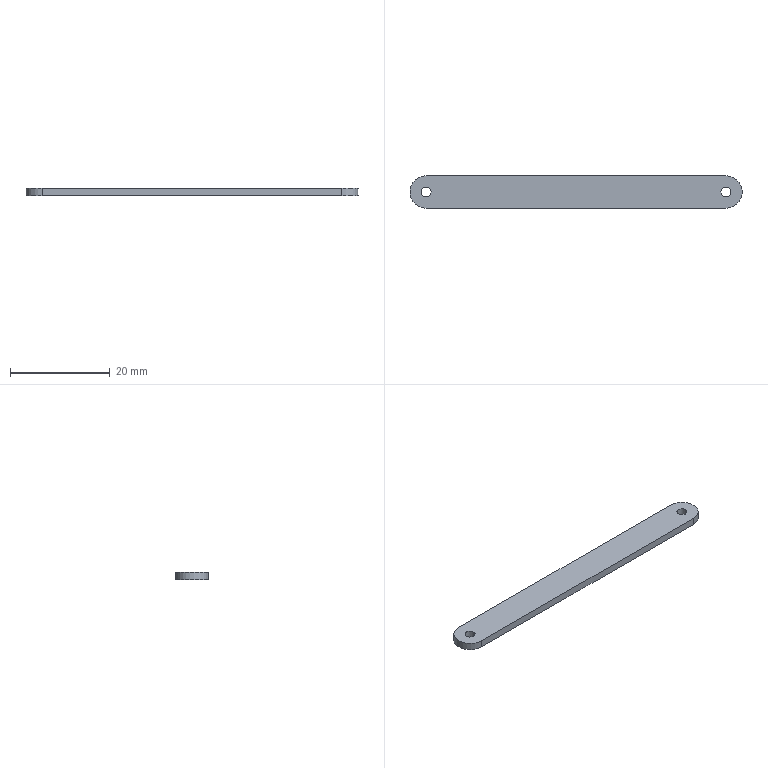Part | NX | features BREP 1 | 1 solid | 8 faces | box 66.5 x 6.5 x 1.5 mm | volume 625.35 mm3 | plane 4 | cylinder 4 | commonest cylinder face diameters 2 x2 6.5 x2
STEP:
#1=CARTESIAN_POINT('',(-29.,0.,0.75));
#2=VERTEX_POINT('',#1);
#3=CARTESIAN_POINT('',(-30.,0.,0.75));
#4=DIRECTION('',(0.,0.,1.));
#5=DIRECTION('',(1.,0.,0.));
#6=AXIS2_PLACEMENT_3D('',#3,#4,#5);
#7=CIRCLE('',#6,1.);
#8=EDGE_CURVE('',#2,#2,#7,.T.);
#9=ORIENTED_EDGE('',*,*,#8,.F.);
#10=EDGE_LOOP('',(#9));
#11=FACE_BOUND('',#10,.T.);
#12=CARTESIAN_POINT('',(-30.,3.25,0.75));
#13=VERTEX_POINT('',#12);
#14=CARTESIAN_POINT('',(-30.,-3.25,0.75));
#15=VERTEX_POINT('',#14);
#16=CARTESIAN_POINT('',(-30.,0.,0.75));
#17=DIRECTION('',(0.,0.,1.));
#18=DIRECTION('',(1.,0.,0.));
#19=AXIS2_PLACEMENT_3D('',#16,#17,#18);
#20=CIRCLE('',#19,3.25);
#21=EDGE_CURVE('',#13,#15,#20,.T.);
#22=ORIENTED_EDGE('',*,*,#21,.T.);
#23=CARTESIAN_POINT('',(30.,-3.25,0.75));
#24=VERTEX_POINT('',#23);
#25=CARTESIAN_POINT('',(-30.,-3.25,0.75));
#26=DIRECTION('',(1.,0.,0.));
#27=VECTOR('',#26,1000.);
#28=LINE('',#25,#27);
#29=EDGE_CURVE('',#15,#24,#28,.T.);
#30=ORIENTED_EDGE('',*,*,#29,.T.);
#31=CARTESIAN_POINT('',(30.,3.25,0.75));
#32=VERTEX_POINT('',#31);
#33=CARTESIAN_POINT('',(30.,0.,0.75));
#34=DIRECTION('',(0.,0.,1.));
#35=DIRECTION('',(1.,0.,0.));
#36=AXIS2_PLACEMENT_3D('',#33,#34,#35);
#37=CIRCLE('',#36,3.25);
#38=EDGE_CURVE('',#24,#32,#37,.T.);
#39=ORIENTED_EDGE('',*,*,#38,.T.);
#40=CARTESIAN_POINT('',(-30.,3.25,0.75));
#41=DIRECTION('',(-1.,0.,0.));
#42=VECTOR('',#41,1000.);
#43=LINE('',#40,#42);
#44=EDGE_CURVE('',#32,#13,#43,.T.);
#45=ORIENTED_EDGE('',*,*,#44,.T.);
#46=EDGE_LOOP('',(#22,#30,#39,#45));
#47=FACE_BOUND('',#46,.T.);
#48=CARTESIAN_POINT('',(31.,0.,0.75));
#49=VERTEX_POINT('',#48);
#50=CARTESIAN_POINT('',(30.,0.,0.75));
#51=DIRECTION('',(0.,0.,1.));
#52=DIRECTION('',(1.,0.,0.));
#53=AXIS2_PLACEMENT_3D('',#50,#51,#52);
#54=CIRCLE('',#53,1.);
#55=EDGE_CURVE('',#49,#49,#54,.T.);
#56=ORIENTED_EDGE('',*,*,#55,.F.);
#57=EDGE_LOOP('',(#56));
#58=FACE_BOUND('',#57,.T.);
#59=CARTESIAN_POINT('',(-30.,0.,0.75));
#60=DIRECTION('',(0.,0.,1.));
#61=DIRECTION('',(-1.,0.,0.));
#62=AXIS2_PLACEMENT_3D('',#59,#60,#61);
#63=PLANE('',#62);
#64=ADVANCED_FACE('',(#11,#47,#58),#63,.T.);
#65=CARTESIAN_POINT('',(-30.,3.25,-0.75));
#66=VERTEX_POINT('',#65);
#67=CARTESIAN_POINT('',(-30.,-3.25,-0.75));
#68=VERTEX_POINT('',#67);
#69=CARTESIAN_POINT('',(-30.,0.,-0.75));
#70=DIRECTION('',(0.,0.,1.));
#71=DIRECTION('',(1.,0.,0.));
#72=AXIS2_PLACEMENT_3D('',#69,#70,#71);
#73=CIRCLE('',#72,3.25);
#74=EDGE_CURVE('',#66,#68,#73,.T.);
#75=ORIENTED_EDGE('',*,*,#74,.F.);
#76=CARTESIAN_POINT('',(30.,3.25,-0.75));
#77=VERTEX_POINT('',#76);
#78=CARTESIAN_POINT('',(-30.,3.25,-0.75));
#79=DIRECTION('',(-1.,0.,0.));
#80=VECTOR('',#79,1000.);
#81=LINE('',#78,#80);
#82=EDGE_CURVE('',#77,#66,#81,.T.);
#83=ORIENTED_EDGE('',*,*,#82,.F.);
#84=CARTESIAN_POINT('',(30.,-3.25,-0.75));
#85=VERTEX_POINT('',#84);
#86=CARTESIAN_POINT('',(30.,0.,-0.75));
#87=DIRECTION('',(0.,0.,1.));
#88=DIRECTION('',(1.,0.,0.));
#89=AXIS2_PLACEMENT_3D('',#86,#87,#88);
#90=CIRCLE('',#89,3.25);
#91=EDGE_CURVE('',#85,#77,#90,.T.);
#92=ORIENTED_EDGE('',*,*,#91,.F.);
#93=CARTESIAN_POINT('',(-30.,-3.25,-0.75));
#94=DIRECTION('',(1.,0.,0.));
#95=VECTOR('',#94,1000.);
#96=LINE('',#93,#95);
#97=EDGE_CURVE('',#68,#85,#96,.T.);
#98=ORIENTED_EDGE('',*,*,#97,.F.);
#99=EDGE_LOOP('',(#75,#83,#92,#98));
#100=FACE_BOUND('',#99,.T.);
#101=CARTESIAN_POINT('',(-29.,0.,-0.75));
#102=VERTEX_POINT('',#101);
#103=CARTESIAN_POINT('',(-30.,0.,-0.75));
#104=DIRECTION('',(0.,0.,1.));
#105=DIRECTION('',(1.,0.,0.));
#106=AXIS2_PLACEMENT_3D('',#103,#104,#105);
#107=CIRCLE('',#106,1.);
#108=EDGE_CURVE('',#102,#102,#107,.T.);
#109=ORIENTED_EDGE('',*,*,#108,.T.);
#110=EDGE_LOOP('',(#109));
#111=FACE_BOUND('',#110,.T.);
#112=CARTESIAN_POINT('',(31.,0.,-0.75));
#113=VERTEX_POINT('',#112);
#114=CARTESIAN_POINT('',(30.,0.,-0.75));
#115=DIRECTION('',(0.,0.,1.));
#116=DIRECTION('',(1.,0.,0.));
#117=AXIS2_PLACEMENT_3D('',#114,#115,#116);
#118=CIRCLE('',#117,1.);
#119=EDGE_CURVE('',#113,#113,#118,.T.);
#120=ORIENTED_EDGE('',*,*,#119,.T.);
#121=EDGE_LOOP('',(#120));
#122=FACE_BOUND('',#121,.T.);
#123=CARTESIAN_POINT('',(-30.,0.,-0.75));
#124=DIRECTION('',(0.,0.,1.));
#125=DIRECTION('',(-1.,0.,0.));
#126=AXIS2_PLACEMENT_3D('',#123,#124,#125);
#127=PLANE('',#126);
#128=ADVANCED_FACE('',(#100,#111,#122),#127,.F.);
#129=ORIENTED_EDGE('',*,*,#74,.T.);
#130=CARTESIAN_POINT('',(-30.,-3.25,0.75));
#131=DIRECTION('',(0.,0.,-1.));
#132=VECTOR('',#131,1000.);
#133=LINE('',#130,#132);
#134=EDGE_CURVE('',#15,#68,#133,.T.);
#135=ORIENTED_EDGE('',*,*,#134,.F.);
#136=ORIENTED_EDGE('',*,*,#21,.F.);
#137=CARTESIAN_POINT('',(-30.,3.25,0.75));
#138=DIRECTION('',(0.,0.,-1.));
#139=VECTOR('',#138,1000.);
#140=LINE('',#137,#139);
#141=EDGE_CURVE('',#13,#66,#140,.T.);
#142=ORIENTED_EDGE('',*,*,#141,.T.);
#143=EDGE_LOOP('',(#129,#135,#136,#142));
#144=FACE_BOUND('',#143,.T.);
#145=CARTESIAN_POINT('',(-30.,0.,0.75));
#146=DIRECTION('',(0.,0.,-1.));
#147=DIRECTION('',(1.,0.,0.));
#148=AXIS2_PLACEMENT_3D('',#145,#146,#147);
#149=CYLINDRICAL_SURFACE('',#148,3.25);
#150=ADVANCED_FACE('',(#144),#149,.T.);
#151=ORIENTED_EDGE('',*,*,#97,.T.);
#152=CARTESIAN_POINT('',(30.,-3.25,0.75));
#153=DIRECTION('',(0.,0.,-1.));
#154=VECTOR('',#153,1000.);
#155=LINE('',#152,#154);
#156=EDGE_CURVE('',#24,#85,#155,.T.);
#157=ORIENTED_EDGE('',*,*,#156,.F.);
#158=ORIENTED_EDGE('',*,*,#29,.F.);
#159=ORIENTED_EDGE('',*,*,#134,.T.);
#160=EDGE_LOOP('',(#151,#157,#158,#159));
#161=FACE_BOUND('',#160,.T.);
#162=CARTESIAN_POINT('',(-30.,-3.25,0.75));
#163=DIRECTION('',(0.,1.,0.));
#164=DIRECTION('',(1.,0.,0.));
#165=AXIS2_PLACEMENT_3D('',#162,#163,#164);
#166=PLANE('',#165);
#167=ADVANCED_FACE('',(#161),#166,.F.);
#168=ORIENTED_EDGE('',*,*,#91,.T.);
#169=CARTESIAN_POINT('',(30.,3.25,0.75));
#170=DIRECTION('',(0.,0.,-1.));
#171=VECTOR('',#170,1000.);
#172=LINE('',#169,#171);
#173=EDGE_CURVE('',#32,#77,#172,.T.);
#174=ORIENTED_EDGE('',*,*,#173,.F.);
#175=ORIENTED_EDGE('',*,*,#38,.F.);
#176=ORIENTED_EDGE('',*,*,#156,.T.);
#177=EDGE_LOOP('',(#168,#174,#175,#176));
#178=FACE_BOUND('',#177,.T.);
#179=CARTESIAN_POINT('',(30.,0.,0.75));
#180=DIRECTION('',(0.,0.,-1.));
#181=DIRECTION('',(1.,0.,0.));
#182=AXIS2_PLACEMENT_3D('',#179,#180,#181);
#183=CYLINDRICAL_SURFACE('',#182,3.25);
#184=ADVANCED_FACE('',(#178),#183,.T.);
#185=ORIENTED_EDGE('',*,*,#82,.T.);
#186=ORIENTED_EDGE('',*,*,#141,.F.);
#187=ORIENTED_EDGE('',*,*,#44,.F.);
#188=ORIENTED_EDGE('',*,*,#173,.T.);
#189=EDGE_LOOP('',(#185,#186,#187,#188));
#190=FACE_BOUND('',#189,.T.);
#191=CARTESIAN_POINT('',(-30.,3.25,0.75));
#192=DIRECTION('',(0.,-1.,0.));
#193=DIRECTION('',(-1.,0.,0.));
#194=AXIS2_PLACEMENT_3D('',#191,#192,#193);
#195=PLANE('',#194);
#196=ADVANCED_FACE('',(#190),#195,.F.);
#197=ORIENTED_EDGE('',*,*,#8,.T.);
#198=EDGE_LOOP('',(#197));
#199=FACE_BOUND('',#198,.T.);
#200=ORIENTED_EDGE('',*,*,#108,.F.);
#201=EDGE_LOOP('',(#200));
#202=FACE_BOUND('',#201,.T.);
#203=CARTESIAN_POINT('',(-30.,0.,0.75));
#204=DIRECTION('',(0.,0.,-1.));
#205=DIRECTION('',(1.,0.,0.));
#206=AXIS2_PLACEMENT_3D('',#203,#204,#205);
#207=CYLINDRICAL_SURFACE('',#206,1.);
#208=ADVANCED_FACE('',(#199,#202),#207,.F.);
#209=ORIENTED_EDGE('',*,*,#55,.T.);
#210=EDGE_LOOP('',(#209));
#211=FACE_BOUND('',#210,.T.);
#212=ORIENTED_EDGE('',*,*,#119,.F.);
#213=EDGE_LOOP('',(#212));
#214=FACE_BOUND('',#213,.T.);
#215=CARTESIAN_POINT('',(30.,0.,0.75));
#216=DIRECTION('',(0.,0.,-1.));
#217=DIRECTION('',(1.,0.,0.));
#218=AXIS2_PLACEMENT_3D('',#215,#216,#217);
#219=CYLINDRICAL_SURFACE('',#218,1.);
#220=ADVANCED_FACE('',(#211,#214),#219,.F.);
#221=CLOSED_SHELL('',(#64,#128,#150,#167,#184,#196,#208,#220));
#222=MANIFOLD_SOLID_BREP('',#221);
#223=(LENGTH_UNIT()NAMED_UNIT(*)SI_UNIT(.MILLI.,.METRE.));
#224=UNCERTAINTY_MEASURE_WITH_UNIT(LENGTH_MEASURE(0.00001),#223,'','');
#225=(NAMED_UNIT(*)PLANE_ANGLE_UNIT()SI_UNIT($,.RADIAN.));
#226=(NAMED_UNIT(*)SI_UNIT($,.STERADIAN.)SOLID_ANGLE_UNIT());
#227=(GEOMETRIC_REPRESENTATION_CONTEXT(3)GLOBAL_UNCERTAINTY_ASSIGNED_CONTEXT((#224))GLOBAL_UNIT_ASSIGNED_CONTEXT((#223,#225,#226))REPRESENTATION_CONTEXT('',''));
#228=ADVANCED_BREP_SHAPE_REPRESENTATION('',(#222),#227);